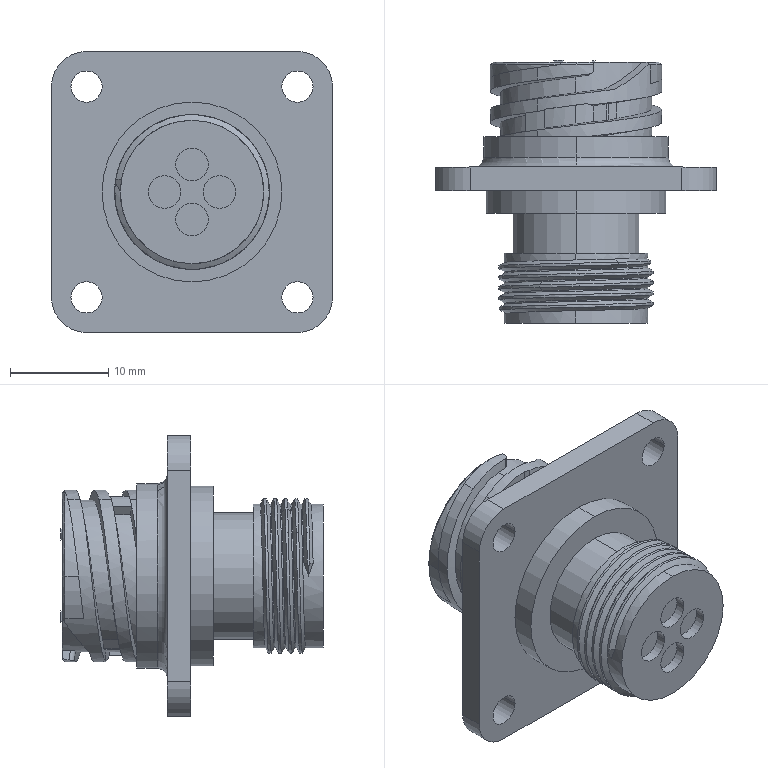Part | SolidWorks | features BaseBody 1 | 1 solid | 201 faces | box 28.575 x 26.721 x 28.575 mm | volume 6118 mm3 | cylinder 99 | plane 75 | spline 14 | cone 7 | torus 6 | commonest cylinder face diameters 3.327 x16 15.73 x12 14.585 x10 3.175 x8 12.852 x8 15.418 x8